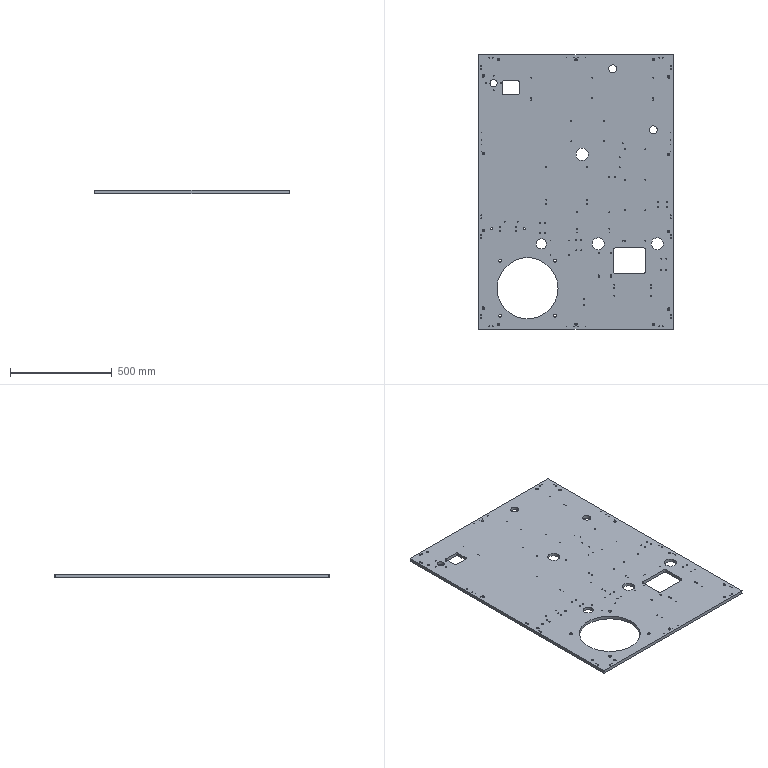Part | STEP file | 2001 Base plate | 1 solid | 410 faces | box 960 x 1350 x 16 mm | volume 18913226 mm3 | cylinder 340 | plane 38 | cone 32 | commonest cylinder face diameters 5 x136 4.2 x44 2.5 x32 7 x28 12 x28 4 x24